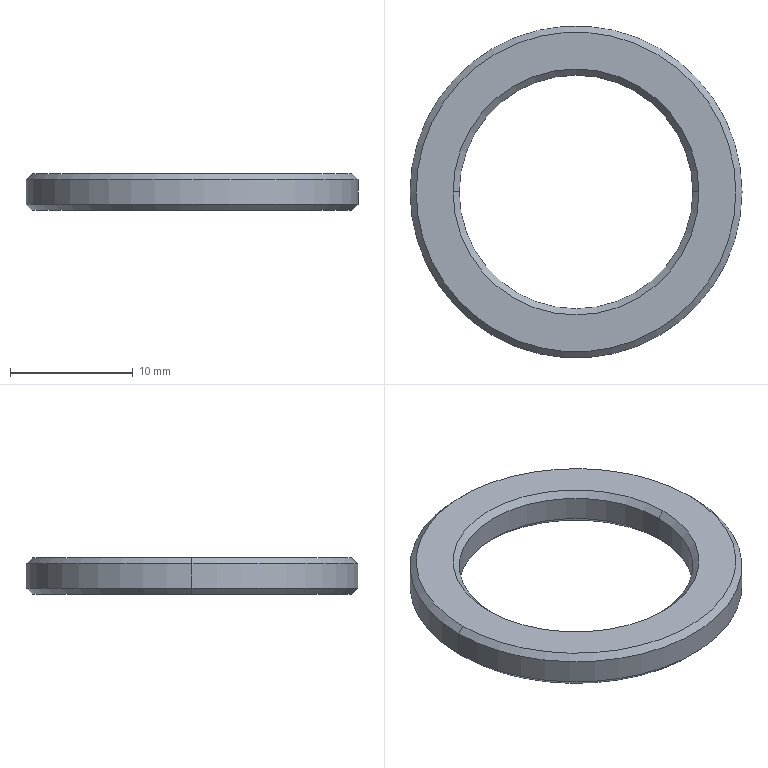Part | STEP file | FWSSS-D27-V19-T3-16 | 1 solid | 14 faces | box 27 x 27 x 3 mm | volume 830.951 mm3 | cone 8 | cylinder 4 | plane 2 | commonest cylinder face diameters 19 x2 27 x2
STEP:
#1=CARTESIAN_POINT('',(0.,0.,0.));
#2=DIRECTION('',(0.,0.,1.));
#3=DIRECTION('',(1.,0.,0.));
#4=AXIS2_PLACEMENT_3D('',#1,#2,#3);
#5=CARTESIAN_POINT('',(9.5,0.,-0.5));
#6=VERTEX_POINT('',#5);
#7=CARTESIAN_POINT('',(10.,0.,0.));
#8=VERTEX_POINT('',#7);
#9=CARTESIAN_POINT('',(10.,0.,0.));
#10=DIRECTION('',(0.7071,0.,0.7071));
#11=VECTOR('',#10,1.);
#12=LINE('',#9,#11);
#13=CARTESIAN_POINT('',(0.,0.,0.));
#14=DIRECTION('',(0.,0.,1.));
#15=DIRECTION('',(1.,0.,0.));
#16=AXIS2_PLACEMENT_3D('',#13,#14,#15);
#17=CONICAL_SURFACE('',#16,10.,0.7854);
#18=CARTESIAN_POINT('',(6.283,0.));
#19=DIRECTION('',(0.,1.));
#20=VECTOR('',#19,1.);
#21=LINE('',#18,#20);
#22=(GEOMETRIC_REPRESENTATION_CONTEXT(2)PARAMETRIC_REPRESENTATION_CONTEXT()REPRESENTATION_CONTEXT('',''));
#23=DEFINITIONAL_REPRESENTATION('',(#21),#22);
#24=PCURVE('',#17,#23);
#25=CARTESIAN_POINT('',(0.,0.,0.));
#26=DIRECTION('',(0.,0.,1.));
#27=DIRECTION('',(1.,0.,0.));
#28=AXIS2_PLACEMENT_3D('',#25,#26,#27);
#29=CONICAL_SURFACE('',#28,10.,0.7854);
#30=CARTESIAN_POINT('',(0.,0.));
#31=DIRECTION('',(0.,1.));
#32=VECTOR('',#31,1.);
#33=LINE('',#30,#32);
#34=(GEOMETRIC_REPRESENTATION_CONTEXT(2)PARAMETRIC_REPRESENTATION_CONTEXT()REPRESENTATION_CONTEXT('',''));
#35=DEFINITIONAL_REPRESENTATION('',(#33),#34);
#36=PCURVE('',#29,#35);
#37=SURFACE_CURVE('',#12,(#24,#36),.PCURVE_S1.);
#38=EDGE_CURVE('',#6,#8,#37,.T.);
#39=ORIENTED_EDGE('',*,*,#38,.T.);
#40=CARTESIAN_POINT('',(-10.,0.,0.));
#41=VERTEX_POINT('',#40);
#42=CARTESIAN_POINT('',(0.,0.,0.));
#43=DIRECTION('',(0.,0.,1.));
#44=DIRECTION('',(1.,0.,0.));
#45=AXIS2_PLACEMENT_3D('',#42,#43,#44);
#46=CIRCLE('',#45,10.);
#47=CARTESIAN_POINT('',(0.,0.));
#48=DIRECTION('',(1.,0.));
#49=VECTOR('',#48,1.);
#50=LINE('',#47,#49);
#51=(GEOMETRIC_REPRESENTATION_CONTEXT(2)PARAMETRIC_REPRESENTATION_CONTEXT()REPRESENTATION_CONTEXT('',''));
#52=DEFINITIONAL_REPRESENTATION('',(#50),#51);
#53=PCURVE('',#17,#52);
#54=CARTESIAN_POINT('',(13.5,0.,0.));
#55=DIRECTION('',(0.,0.,-1.));
#56=DIRECTION('',(-1.,0.,0.));
#57=AXIS2_PLACEMENT_3D('',#54,#55,#56);
#58=PLANE('',#57);
#59=CARTESIAN_POINT('',(3.5,0.));
#60=CARTESIAN_POINT('',(3.5,17.321));
#61=CARTESIAN_POINT('',(18.5,8.66));
#62=CARTESIAN_POINT('',(33.5,0.));
#63=CARTESIAN_POINT('',(18.5,-8.66));
#64=CARTESIAN_POINT('',(3.5,-17.321));
#65=CARTESIAN_POINT('',(3.5,0.));
#66=(BOUNDED_CURVE()B_SPLINE_CURVE(2,(#59,#60,#61,#62,#63,#64,#65),.UNSPECIFIED.,.T.,.F.)B_SPLINE_CURVE_WITH_KNOTS((1,2,2,2,2,1),(-2.094,0.,2.094,4.189,6.283,8.378),.UNSPECIFIED.)CURVE()GEOMETRIC_REPRESENTATION_ITEM()RATIONAL_B_SPLINE_CURVE((1.,0.5,1.,0.5,1.,0.5,1.))REPRESENTATION_ITEM(''));
#67=(GEOMETRIC_REPRESENTATION_CONTEXT(2)PARAMETRIC_REPRESENTATION_CONTEXT()REPRESENTATION_CONTEXT('',''));
#68=DEFINITIONAL_REPRESENTATION('',(#66),#67);
#69=PCURVE('',#58,#68);
#70=SURFACE_CURVE('',#46,(#53,#69),.PCURVE_S1.);
#71=EDGE_CURVE('',#41,#8,#70,.T.);
#72=ORIENTED_EDGE('',*,*,#71,.F.);
#73=CARTESIAN_POINT('',(-9.5,0.,-0.5));
#74=VERTEX_POINT('',#73);
#75=CARTESIAN_POINT('',(-10.,0.,0.));
#76=DIRECTION('',(-0.7071,0.,0.7071));
#77=VECTOR('',#76,1.);
#78=LINE('',#75,#77);
#79=CARTESIAN_POINT('',(3.142,0.));
#80=DIRECTION('',(0.,1.));
#81=VECTOR('',#80,1.);
#82=LINE('',#79,#81);
#83=(GEOMETRIC_REPRESENTATION_CONTEXT(2)PARAMETRIC_REPRESENTATION_CONTEXT()REPRESENTATION_CONTEXT('',''));
#84=DEFINITIONAL_REPRESENTATION('',(#82),#83);
#85=PCURVE('',#17,#84);
#86=CARTESIAN_POINT('',(3.142,0.));
#87=DIRECTION('',(0.,1.));
#88=VECTOR('',#87,1.);
#89=LINE('',#86,#88);
#90=(GEOMETRIC_REPRESENTATION_CONTEXT(2)PARAMETRIC_REPRESENTATION_CONTEXT()REPRESENTATION_CONTEXT('',''));
#91=DEFINITIONAL_REPRESENTATION('',(#89),#90);
#92=PCURVE('',#29,#91);
#93=SURFACE_CURVE('',#78,(#85,#92),.PCURVE_S1.);
#94=EDGE_CURVE('',#74,#41,#93,.T.);
#95=ORIENTED_EDGE('',*,*,#94,.F.);
#96=CARTESIAN_POINT('',(0.,0.,-0.5));
#97=DIRECTION('',(0.,0.,1.));
#98=DIRECTION('',(1.,0.,0.));
#99=AXIS2_PLACEMENT_3D('',#96,#97,#98);
#100=CIRCLE('',#99,9.5);
#101=CARTESIAN_POINT('',(0.,-0.5));
#102=DIRECTION('',(1.,0.));
#103=VECTOR('',#102,1.);
#104=LINE('',#101,#103);
#105=(GEOMETRIC_REPRESENTATION_CONTEXT(2)PARAMETRIC_REPRESENTATION_CONTEXT()REPRESENTATION_CONTEXT('',''));
#106=DEFINITIONAL_REPRESENTATION('',(#104),#105);
#107=PCURVE('',#17,#106);
#108=CARTESIAN_POINT('',(0.,0.,0.));
#109=DIRECTION('',(0.,0.,1.));
#110=DIRECTION('',(1.,0.,0.));
#111=AXIS2_PLACEMENT_3D('',#108,#109,#110);
#112=CYLINDRICAL_SURFACE('',#111,9.5);
#113=CARTESIAN_POINT('',(0.,-0.5));
#114=DIRECTION('',(1.,0.));
#115=VECTOR('',#114,1.);
#116=LINE('',#113,#115);
#117=(GEOMETRIC_REPRESENTATION_CONTEXT(2)PARAMETRIC_REPRESENTATION_CONTEXT()REPRESENTATION_CONTEXT('',''));
#118=DEFINITIONAL_REPRESENTATION('',(#116),#117);
#119=PCURVE('',#112,#118);
#120=SURFACE_CURVE('',#100,(#107,#119),.PCURVE_S1.);
#121=EDGE_CURVE('',#74,#6,#120,.T.);
#122=ORIENTED_EDGE('',*,*,#121,.T.);
#123=EDGE_LOOP('',(#39,#72,#95,#122));
#124=FACE_BOUND('',#123,.F.);
#125=ADVANCED_FACE('',(#124),#17,.F.);
#126=CARTESIAN_POINT('',(-9.5,0.,-2.5));
#127=VERTEX_POINT('',#126);
#128=CARTESIAN_POINT('',(-10.,0.,-3.));
#129=VERTEX_POINT('',#128);
#130=CARTESIAN_POINT('',(-9.5,0.,-2.5));
#131=DIRECTION('',(-0.7071,0.,-0.7071));
#132=VECTOR('',#131,1.);
#133=LINE('',#130,#132);
#134=CARTESIAN_POINT('',(0.,0.,-2.5));
#135=DIRECTION('',(0.,0.,-1.));
#136=DIRECTION('',(-1.,0.,0.));
#137=AXIS2_PLACEMENT_3D('',#134,#135,#136);
#138=CONICAL_SURFACE('',#137,9.5,0.7854);
#139=CARTESIAN_POINT('',(6.283,0.));
#140=DIRECTION('',(0.,1.));
#141=VECTOR('',#140,1.);
#142=LINE('',#139,#141);
#143=(GEOMETRIC_REPRESENTATION_CONTEXT(2)PARAMETRIC_REPRESENTATION_CONTEXT()REPRESENTATION_CONTEXT('',''));
#144=DEFINITIONAL_REPRESENTATION('',(#142),#143);
#145=PCURVE('',#138,#144);
#146=CARTESIAN_POINT('',(0.,0.,-2.5));
#147=DIRECTION('',(0.,0.,-1.));
#148=DIRECTION('',(-1.,0.,0.));
#149=AXIS2_PLACEMENT_3D('',#146,#147,#148);
#150=CONICAL_SURFACE('',#149,9.5,0.7854);
#151=CARTESIAN_POINT('',(0.,0.));
#152=DIRECTION('',(0.,1.));
#153=VECTOR('',#152,1.);
#154=LINE('',#151,#153);
#155=(GEOMETRIC_REPRESENTATION_CONTEXT(2)PARAMETRIC_REPRESENTATION_CONTEXT()REPRESENTATION_CONTEXT('',''));
#156=DEFINITIONAL_REPRESENTATION('',(#154),#155);
#157=PCURVE('',#150,#156);
#158=SURFACE_CURVE('',#133,(#145,#157),.PCURVE_S1.);
#159=EDGE_CURVE('',#127,#129,#158,.T.);
#160=ORIENTED_EDGE('',*,*,#159,.T.);
#161=CARTESIAN_POINT('',(10.,0.,-3.));
#162=VERTEX_POINT('',#161);
#163=CARTESIAN_POINT('',(0.,0.,-3.));
#164=DIRECTION('',(0.,0.,1.));
#165=DIRECTION('',(1.,0.,0.));
#166=AXIS2_PLACEMENT_3D('',#163,#164,#165);
#167=CIRCLE('',#166,10.);
#168=CARTESIAN_POINT('',(9.425,0.5));
#169=DIRECTION('',(-1.,0.));
#170=VECTOR('',#169,1.);
#171=LINE('',#168,#170);
#172=(GEOMETRIC_REPRESENTATION_CONTEXT(2)PARAMETRIC_REPRESENTATION_CONTEXT()REPRESENTATION_CONTEXT('',''));
#173=DEFINITIONAL_REPRESENTATION('',(#171),#172);
#174=PCURVE('',#138,#173);
#175=CARTESIAN_POINT('',(0.,0.,-3.));
#176=DIRECTION('',(0.,0.,1.));
#177=DIRECTION('',(1.,0.,0.));
#178=AXIS2_PLACEMENT_3D('',#175,#176,#177);
#179=PLANE('',#178);
#180=CARTESIAN_POINT('',(0.,0.));
#181=DIRECTION('',(1.,0.));
#182=AXIS2_PLACEMENT_2D('',#180,#181);
#183=CIRCLE('',#182,10.);
#184=(GEOMETRIC_REPRESENTATION_CONTEXT(2)PARAMETRIC_REPRESENTATION_CONTEXT()REPRESENTATION_CONTEXT('',''));
#185=DEFINITIONAL_REPRESENTATION('',(#183),#184);
#186=PCURVE('',#179,#185);
#187=SURFACE_CURVE('',#167,(#174,#186),.PCURVE_S1.);
#188=EDGE_CURVE('',#129,#162,#187,.T.);
#189=ORIENTED_EDGE('',*,*,#188,.T.);
#190=CARTESIAN_POINT('',(9.5,0.,-2.5));
#191=VERTEX_POINT('',#190);
#192=CARTESIAN_POINT('',(9.5,0.,-2.5));
#193=DIRECTION('',(0.7071,0.,-0.7071));
#194=VECTOR('',#193,1.);
#195=LINE('',#192,#194);
#196=CARTESIAN_POINT('',(3.142,0.));
#197=DIRECTION('',(0.,1.));
#198=VECTOR('',#197,1.);
#199=LINE('',#196,#198);
#200=(GEOMETRIC_REPRESENTATION_CONTEXT(2)PARAMETRIC_REPRESENTATION_CONTEXT()REPRESENTATION_CONTEXT('',''));
#201=DEFINITIONAL_REPRESENTATION('',(#199),#200);
#202=PCURVE('',#138,#201);
#203=CARTESIAN_POINT('',(3.142,0.));
#204=DIRECTION('',(0.,1.));
#205=VECTOR('',#204,1.);
#206=LINE('',#203,#205);
#207=(GEOMETRIC_REPRESENTATION_CONTEXT(2)PARAMETRIC_REPRESENTATION_CONTEXT()REPRESENTATION_CONTEXT('',''));
#208=DEFINITIONAL_REPRESENTATION('',(#206),#207);
#209=PCURVE('',#150,#208);
#210=SURFACE_CURVE('',#195,(#202,#209),.PCURVE_S1.);
#211=EDGE_CURVE('',#191,#162,#210,.T.);
#212=ORIENTED_EDGE('',*,*,#211,.F.);
#213=CARTESIAN_POINT('',(0.,0.,-2.5));
#214=DIRECTION('',(0.,0.,1.));
#215=DIRECTION('',(1.,0.,0.));
#216=AXIS2_PLACEMENT_3D('',#213,#214,#215);
#217=CIRCLE('',#216,9.5);
#218=CARTESIAN_POINT('',(9.425,0.));
#219=DIRECTION('',(-1.,0.));
#220=VECTOR('',#219,1.);
#221=LINE('',#218,#220);
#222=(GEOMETRIC_REPRESENTATION_CONTEXT(2)PARAMETRIC_REPRESENTATION_CONTEXT()REPRESENTATION_CONTEXT('',''));
#223=DEFINITIONAL_REPRESENTATION('',(#221),#222);
#224=PCURVE('',#138,#223);
#225=CARTESIAN_POINT('',(0.,-2.5));
#226=DIRECTION('',(1.,0.));
#227=VECTOR('',#226,1.);
#228=LINE('',#225,#227);
#229=(GEOMETRIC_REPRESENTATION_CONTEXT(2)PARAMETRIC_REPRESENTATION_CONTEXT()REPRESENTATION_CONTEXT('',''));
#230=DEFINITIONAL_REPRESENTATION('',(#228),#229);
#231=PCURVE('',#112,#230);
#232=SURFACE_CURVE('',#217,(#224,#231),.PCURVE_S1.);
#233=EDGE_CURVE('',#127,#191,#232,.T.);
#234=ORIENTED_EDGE('',*,*,#233,.F.);
#235=EDGE_LOOP('',(#160,#189,#212,#234));
#236=FACE_BOUND('',#235,.F.);
#237=ADVANCED_FACE('',(#236),#138,.F.);
#238=CARTESIAN_POINT('',(9.5,0.,0.));
#239=DIRECTION('',(0.,0.,1.));
#240=VECTOR('',#239,1.);
#241=LINE('',#238,#240);
#242=CARTESIAN_POINT('',(6.283,0.));
#243=DIRECTION('',(0.,1.));
#244=VECTOR('',#243,1.);
#245=LINE('',#242,#244);
#246=(GEOMETRIC_REPRESENTATION_CONTEXT(2)PARAMETRIC_REPRESENTATION_CONTEXT()REPRESENTATION_CONTEXT('',''));
#247=DEFINITIONAL_REPRESENTATION('',(#245),#246);
#248=PCURVE('',#112,#247);
#249=CARTESIAN_POINT('',(0.,0.,0.));
#250=DIRECTION('',(0.,0.,1.));
#251=DIRECTION('',(1.,0.,0.));
#252=AXIS2_PLACEMENT_3D('',#249,#250,#251);
#253=CYLINDRICAL_SURFACE('',#252,9.5);
#254=CARTESIAN_POINT('',(0.,0.));
#255=DIRECTION('',(0.,1.));
#256=VECTOR('',#255,1.);
#257=LINE('',#254,#256);
#258=(GEOMETRIC_REPRESENTATION_CONTEXT(2)PARAMETRIC_REPRESENTATION_CONTEXT()REPRESENTATION_CONTEXT('',''));
#259=DEFINITIONAL_REPRESENTATION('',(#257),#258);
#260=PCURVE('',#253,#259);
#261=SURFACE_CURVE('',#241,(#248,#260),.PCURVE_S1.);
#262=EDGE_CURVE('',#191,#6,#261,.T.);
#263=ORIENTED_EDGE('',*,*,#262,.T.);
#264=ORIENTED_EDGE('',*,*,#121,.F.);
#265=CARTESIAN_POINT('',(-9.5,0.,0.));
#266=DIRECTION('',(0.,0.,1.));
#267=VECTOR('',#266,1.);
#268=LINE('',#265,#267);
#269=CARTESIAN_POINT('',(3.142,0.));
#270=DIRECTION('',(0.,1.));
#271=VECTOR('',#270,1.);
#272=LINE('',#269,#271);
#273=(GEOMETRIC_REPRESENTATION_CONTEXT(2)PARAMETRIC_REPRESENTATION_CONTEXT()REPRESENTATION_CONTEXT('',''));
#274=DEFINITIONAL_REPRESENTATION('',(#272),#273);
#275=PCURVE('',#112,#274);
#276=CARTESIAN_POINT('',(3.142,0.));
#277=DIRECTION('',(0.,1.));
#278=VECTOR('',#277,1.);
#279=LINE('',#276,#278);
#280=(GEOMETRIC_REPRESENTATION_CONTEXT(2)PARAMETRIC_REPRESENTATION_CONTEXT()REPRESENTATION_CONTEXT('',''));
#281=DEFINITIONAL_REPRESENTATION('',(#279),#280);
#282=PCURVE('',#253,#281);
#283=SURFACE_CURVE('',#268,(#275,#282),.PCURVE_S1.);
#284=EDGE_CURVE('',#127,#74,#283,.T.);
#285=ORIENTED_EDGE('',*,*,#284,.F.);
#286=ORIENTED_EDGE('',*,*,#233,.T.);
#287=EDGE_LOOP('',(#263,#264,#285,#286));
#288=FACE_BOUND('',#287,.F.);
#289=ADVANCED_FACE('',(#288),#112,.F.);
#290=CARTESIAN_POINT('',(13.,0.,0.));
#291=VERTEX_POINT('',#290);
#292=CARTESIAN_POINT('',(-13.,0.,0.));
#293=VERTEX_POINT('',#292);
#294=CARTESIAN_POINT('',(0.,0.,0.));
#295=DIRECTION('',(0.,0.,1.));
#296=DIRECTION('',(1.,0.,0.));
#297=AXIS2_PLACEMENT_3D('',#294,#295,#296);
#298=CIRCLE('',#297,13.);
#299=CARTESIAN_POINT('',(0.,0.,-0.5));
#300=DIRECTION('',(0.,0.,-1.));
#301=DIRECTION('',(-1.,0.,0.));
#302=AXIS2_PLACEMENT_3D('',#299,#300,#301);
#303=CONICAL_SURFACE('',#302,13.5,0.7854);
#304=CARTESIAN_POINT('',(3.142,-0.5));
#305=DIRECTION('',(-1.,0.));
#306=VECTOR('',#305,1.);
#307=LINE('',#304,#306);
#308=(GEOMETRIC_REPRESENTATION_CONTEXT(2)PARAMETRIC_REPRESENTATION_CONTEXT()REPRESENTATION_CONTEXT('',''));
#309=DEFINITIONAL_REPRESENTATION('',(#307),#308);
#310=PCURVE('',#303,#309);
#311=CARTESIAN_POINT('',(0.5,0.));
#312=CARTESIAN_POINT('',(0.5,22.517));
#313=CARTESIAN_POINT('',(20.,11.258));
#314=CARTESIAN_POINT('',(39.5,0.));
#315=CARTESIAN_POINT('',(20.,-11.258));
#316=CARTESIAN_POINT('',(0.5,-22.517));
#317=CARTESIAN_POINT('',(0.5,0.));
#318=(BOUNDED_CURVE()B_SPLINE_CURVE(2,(#311,#312,#313,#314,#315,#316,#317),.UNSPECIFIED.,.T.,.F.)B_SPLINE_CURVE_WITH_KNOTS((1,2,2,2,2,1),(-2.094,0.,2.094,4.189,6.283,8.378),.UNSPECIFIED.)CURVE()GEOMETRIC_REPRESENTATION_ITEM()RATIONAL_B_SPLINE_CURVE((1.,0.5,1.,0.5,1.,0.5,1.))REPRESENTATION_ITEM(''));
#319=(GEOMETRIC_REPRESENTATION_CONTEXT(2)PARAMETRIC_REPRESENTATION_CONTEXT()REPRESENTATION_CONTEXT('',''));
#320=DEFINITIONAL_REPRESENTATION('',(#318),#319);
#321=PCURVE('',#58,#320);
#322=SURFACE_CURVE('',#298,(#310,#321),.PCURVE_S1.);
#323=EDGE_CURVE('',#291,#293,#322,.T.);
#324=ORIENTED_EDGE('',*,*,#323,.F.);
#325=CARTESIAN_POINT('',(13.5,0.,-0.5));
#326=VERTEX_POINT('',#325);
#327=CARTESIAN_POINT('',(13.5,0.,-0.5));
#328=DIRECTION('',(0.7071,0.,-0.7071));
#329=VECTOR('',#328,1.);
#330=LINE('',#327,#329);
#331=CARTESIAN_POINT('',(3.142,0.));
#332=DIRECTION('',(0.,1.));
#333=VECTOR('',#332,1.);
#334=LINE('',#331,#333);
#335=(GEOMETRIC_REPRESENTATION_CONTEXT(2)PARAMETRIC_REPRESENTATION_CONTEXT()REPRESENTATION_CONTEXT('',''));
#336=DEFINITIONAL_REPRESENTATION('',(#334),#335);
#337=PCURVE('',#303,#336);
#338=CARTESIAN_POINT('',(0.,0.,-0.5));
#339=DIRECTION('',(0.,0.,-1.));
#340=DIRECTION('',(-1.,0.,0.));
#341=AXIS2_PLACEMENT_3D('',#338,#339,#340);
#342=CONICAL_SURFACE('',#341,13.5,0.7854);
#343=CARTESIAN_POINT('',(3.142,0.));
#344=DIRECTION('',(0.,1.));
#345=VECTOR('',#344,1.);
#346=LINE('',#343,#345);
#347=(GEOMETRIC_REPRESENTATION_CONTEXT(2)PARAMETRIC_REPRESENTATION_CONTEXT()REPRESENTATION_CONTEXT('',''));
#348=DEFINITIONAL_REPRESENTATION('',(#346),#347);
#349=PCURVE('',#342,#348);
#350=SURFACE_CURVE('',#330,(#337,#349),.PCURVE_S1.);
#351=EDGE_CURVE('',#291,#326,#350,.T.);
#352=ORIENTED_EDGE('',*,*,#351,.T.);
#353=CARTESIAN_POINT('',(-13.5,0.,-0.5));
#354=VERTEX_POINT('',#353);
#355=CARTESIAN_POINT('',(0.,0.,-0.5));
#356=DIRECTION('',(0.,0.,1.));
#357=DIRECTION('',(1.,0.,0.));
#358=AXIS2_PLACEMENT_3D('',#355,#356,#357);
#359=CIRCLE('',#358,13.5);
#360=CARTESIAN_POINT('',(3.142,0.));
#361=DIRECTION('',(-1.,0.));
#362=VECTOR('',#361,1.);
#363=LINE('',#360,#362);
#364=(GEOMETRIC_REPRESENTATION_CONTEXT(2)PARAMETRIC_REPRESENTATION_CONTEXT()REPRESENTATION_CONTEXT('',''));
#365=DEFINITIONAL_REPRESENTATION('',(#363),#364);
#366=PCURVE('',#303,#365);
#367=CARTESIAN_POINT('',(0.,0.,0.));
#368=DIRECTION('',(0.,0.,1.));
#369=DIRECTION('',(1.,0.,0.));
#370=AXIS2_PLACEMENT_3D('',#367,#368,#369);
#371=CYLINDRICAL_SURFACE('',#370,13.5);
#372=CARTESIAN_POINT('',(0.,-0.5));
#373=DIRECTION('',(1.,0.));
#374=VECTOR('',#373,1.);
#375=LINE('',#372,#374);
#376=(GEOMETRIC_REPRESENTATION_CONTEXT(2)PARAMETRIC_REPRESENTATION_CONTEXT()REPRESENTATION_CONTEXT('',''));
#377=DEFINITIONAL_REPRESENTATION('',(#375),#376);
#378=PCURVE('',#371,#377);
#379=SURFACE_CURVE('',#359,(#366,#378),.PCURVE_S1.);
#380=EDGE_CURVE('',#326,#354,#379,.T.);
#381=ORIENTED_EDGE('',*,*,#380,.T.);
#382=CARTESIAN_POINT('',(-13.5,0.,-0.5));
#383=DIRECTION('',(-0.7071,0.,-0.7071));
#384=VECTOR('',#383,1.);
#385=LINE('',#382,#384);
#386=CARTESIAN_POINT('',(0.,0.));
#387=DIRECTION('',(0.,1.));
#388=VECTOR('',#387,1.);
#389=LINE('',#386,#388);
#390=(GEOMETRIC_REPRESENTATION_CONTEXT(2)PARAMETRIC_REPRESENTATION_CONTEXT()REPRESENTATION_CONTEXT('',''));
#391=DEFINITIONAL_REPRESENTATION('',(#389),#390);
#392=PCURVE('',#303,#391);
#393=CARTESIAN_POINT('',(6.283,0.));
#394=DIRECTION('',(0.,1.));
#395=VECTOR('',#394,1.);
#396=LINE('',#393,#395);
#397=(GEOMETRIC_REPRESENTATION_CONTEXT(2)PARAMETRIC_REPRESENTATION_CONTEXT()REPRESENTATION_CONTEXT('',''));
#398=DEFINITIONAL_REPRESENTATION('',(#396),#397);
#399=PCURVE('',#342,#398);
#400=SURFACE_CURVE('',#385,(#392,#399),.PCURVE_S1.);
#401=EDGE_CURVE('',#293,#354,#400,.T.);
#402=ORIENTED_EDGE('',*,*,#401,.F.);
#403=EDGE_LOOP('',(#324,#352,#381,#402));
#404=FACE_BOUND('',#403,.T.);
#405=ADVANCED_FACE('',(#404),#303,.T.);
#406=CARTESIAN_POINT('',(13.,0.,-3.));
#407=VERTEX_POINT('',#406);
#408=CARTESIAN_POINT('',(-13.,0.,-3.));
#409=VERTEX_POINT('',#408);
#410=CARTESIAN_POINT('',(0.,0.,-3.));
#411=DIRECTION('',(0.,0.,1.));
#412=DIRECTION('',(1.,0.,0.));
#413=AXIS2_PLACEMENT_3D('',#410,#411,#412);
#414=CIRCLE('',#413,13.);
#415=CARTESIAN_POINT('',(0.,0.,-3.));
#416=DIRECTION('',(0.,0.,1.));
#417=DIRECTION('',(1.,0.,0.));
#418=AXIS2_PLACEMENT_3D('',#415,#416,#417);
#419=CONICAL_SURFACE('',#418,13.,0.7854);
#420=CARTESIAN_POINT('',(0.,0.));
#421=DIRECTION('',(1.,0.));
#422=VECTOR('',#421,1.);
#423=LINE('',#420,#422);
#424=(GEOMETRIC_REPRESENTATION_CONTEXT(2)PARAMETRIC_REPRESENTATION_CONTEXT()REPRESENTATION_CONTEXT('',''));
#425=DEFINITIONAL_REPRESENTATION('',(#423),#424);
#426=PCURVE('',#419,#425);
#427=CARTESIAN_POINT('',(0.,0.));
#428=DIRECTION('',(1.,0.));
#429=AXIS2_PLACEMENT_2D('',#427,#428);
#430=CIRCLE('',#429,13.);
#431=(GEOMETRIC_REPRESENTATION_CONTEXT(2)PARAMETRIC_REPRESENTATION_CONTEXT()REPRESENTATION_CONTEXT('',''));
#432=DEFINITIONAL_REPRESENTATION('',(#430),#431);
#433=PCURVE('',#179,#432);
#434=SURFACE_CURVE('',#414,(#426,#433),.PCURVE_S1.);
#435=EDGE_CURVE('',#407,#409,#434,.T.);
#436=ORIENTED_EDGE('',*,*,#435,.T.);
#437=CARTESIAN_POINT('',(-13.5,0.,-2.5));
#438=VERTEX_POINT('',#437);
#439=CARTESIAN_POINT('',(-13.,0.,-3.));
#440=DIRECTION('',(-0.7071,0.,0.7071));
#441=VECTOR('',#440,1.);
#442=LINE('',#439,#441);
#443=CARTESIAN_POINT('',(3.142,0.));
#444=DIRECTION('',(0.,1.));
#445=VECTOR('',#444,1.);
#446=LINE('',#443,#445);
#447=(GEOMETRIC_REPRESENTATION_CONTEXT(2)PARAMETRIC_REPRESENTATION_CONTEXT()REPRESENTATION_CONTEXT('',''));
#448=DEFINITIONAL_REPRESENTATION('',(#446),#447);
#449=PCURVE('',#419,#448);
#450=CARTESIAN_POINT('',(0.,0.,-3.));
#451=DIRECTION('',(0.,0.,1.));
#452=DIRECTION('',(1.,0.,0.));
#453=AXIS2_PLACEMENT_3D('',#450,#451,#452);
#454=CONICAL_SURFACE('',#453,13.,0.7854);
#455=CARTESIAN_POINT('',(3.142,0.));
#456=DIRECTION('',(0.,1.));
#457=VECTOR('',#456,1.);
#458=LINE('',#455,#457);
#459=(GEOMETRIC_REPRESENTATION_CONTEXT(2)PARAMETRIC_REPRESENTATION_CONTEXT()REPRESENTATION_CONTEXT('',''));
#460=DEFINITIONAL_REPRESENTATION('',(#458),#459);
#461=PCURVE('',#454,#460);
#462=SURFACE_CURVE('',#442,(#449,#461),.PCURVE_S1.);
#463=EDGE_CURVE('',#409,#438,#462,.T.);
#464=ORIENTED_EDGE('',*,*,#463,.T.);
#465=CARTESIAN_POINT('',(13.5,0.,-2.5));
#466=VERTEX_POINT('',#465);
#467=CARTESIAN_POINT('',(0.,0.,-2.5));
#468=DIRECTION('',(0.,0.,1.));
#469=DIRECTION('',(1.,0.,0.));
#470=AXIS2_PLACEMENT_3D('',#467,#468,#469);
#471=CIRCLE('',#470,13.5);
#472=CARTESIAN_POINT('',(0.,0.5));
#473=DIRECTION('',(1.,0.));
#474=VECTOR('',#473,1.);
#475=LINE('',#472,#474);
#476=(GEOMETRIC_REPRESENTATION_CONTEXT(2)PARAMETRIC_REPRESENTATION_CONTEXT()REPRESENTATION_CONTEXT('',''));
#477=DEFINITIONAL_REPRESENTATION('',(#475),#476);
#478=PCURVE('',#419,#477);
#479=CARTESIAN_POINT('',(0.,-2.5));
#480=DIRECTION('',(1.,0.));
#481=VECTOR('',#480,1.);
#482=LINE('',#479,#481);
#483=(GEOMETRIC_REPRESENTATION_CONTEXT(2)PARAMETRIC_REPRESENTATION_CONTEXT()REPRESENTATION_CONTEXT('',''));
#484=DEFINITIONAL_REPRESENTATION('',(#482),#483);
#485=PCURVE('',#371,#484);
#486=SURFACE_CURVE('',#471,(#478,#485),.PCURVE_S1.);
#487=EDGE_CURVE('',#466,#438,#486,.T.);
#488=ORIENTED_EDGE('',*,*,#487,.F.);
#489=CARTESIAN_POINT('',(13.,0.,-3.));
#490=DIRECTION('',(0.7071,0.,0.7071));
#491=VECTOR('',#490,1.);
#492=LINE('',#489,#491);
#493=CARTESIAN_POINT('',(0.,0.));
#494=DIRECTION('',(0.,1.));
#495=VECTOR('',#494,1.);
#496=LINE('',#493,#495);
#497=(GEOMETRIC_REPRESENTATION_CONTEXT(2)PARAMETRIC_REPRESENTATION_CONTEXT()REPRESENTATION_CONTEXT('',''));
#498=DEFINITIONAL_REPRESENTATION('',(#496),#497);
#499=PCURVE('',#419,#498);
#500=CARTESIAN_POINT('',(6.283,0.));
#501=DIRECTION('',(0.,1.));
#502=VECTOR('',#501,1.);
#503=LINE('',#500,#502);
#504=(GEOMETRIC_REPRESENTATION_CONTEXT(2)PARAMETRIC_REPRESENTATION_CONTEXT()REPRESENTATION_CONTEXT('',''));
#505=DEFINITIONAL_REPRESENTATION('',(#503),#504);
#506=PCURVE('',#454,#505);
#507=SURFACE_CURVE('',#492,(#499,#506),.PCURVE_S1.);
#508=EDGE_CURVE('',#407,#466,#507,.T.);
#509=ORIENTED_EDGE('',*,*,#508,.F.);
#510=EDGE_LOOP('',(#436,#464,#488,#509));
#511=FACE_BOUND('',#510,.T.);
#512=ADVANCED_FACE('',(#511),#419,.T.);
#513=ORIENTED_EDGE('',*,*,#487,.T.);
#514=CARTESIAN_POINT('',(-13.5,0.,0.));
#515=DIRECTION('',(0.,0.,1.));
#516=VECTOR('',#515,1.);
#517=LINE('',#514,#516);
#518=CARTESIAN_POINT('',(3.142,0.));
#519=DIRECTION('',(0.,1.));
#520=VECTOR('',#519,1.);
#521=LINE('',#518,#520);
#522=(GEOMETRIC_REPRESENTATION_CONTEXT(2)PARAMETRIC_REPRESENTATION_CONTEXT()REPRESENTATION_CONTEXT('',''));
#523=DEFINITIONAL_REPRESENTATION('',(#521),#522);
#524=PCURVE('',#371,#523);
#525=CARTESIAN_POINT('',(0.,0.,0.));
#526=DIRECTION('',(0.,0.,1.));
#527=DIRECTION('',(1.,0.,0.));
#528=AXIS2_PLACEMENT_3D('',#525,#526,#527);
#529=CYLINDRICAL_SURFACE('',#528,13.5);
#530=CARTESIAN_POINT('',(3.142,0.));
#531=DIRECTION('',(0.,1.));
#532=VECTOR('',#531,1.);
#533=LINE('',#530,#532);
#534=(GEOMETRIC_REPRESENTATION_CONTEXT(2)PARAMETRIC_REPRESENTATION_CONTEXT()REPRESENTATION_CONTEXT('',''));
#535=DEFINITIONAL_REPRESENTATION('',(#533),#534);
#536=PCURVE('',#529,#535);
#537=SURFACE_CURVE('',#517,(#524,#536),.PCURVE_S1.);
#538=EDGE_CURVE('',#438,#354,#537,.T.);
#539=ORIENTED_EDGE('',*,*,#538,.T.);
#540=ORIENTED_EDGE('',*,*,#380,.F.);
#541=CARTESIAN_POINT('',(13.5,0.,0.));
#542=DIRECTION('',(0.,0.,1.));
#543=VECTOR('',#542,1.);
#544=LINE('',#541,#543);
#545=CARTESIAN_POINT('',(0.,0.));
#546=DIRECTION('',(0.,1.));
#547=VECTOR('',#546,1.);
#548=LINE('',#545,#547);
#549=(GEOMETRIC_REPRESENTATION_CONTEXT(2)PARAMETRIC_REPRESENTATION_CONTEXT()REPRESENTATION_CONTEXT('',''));
#550=DEFINITIONAL_REPRESENTATION('',(#548),#549);
#551=PCURVE('',#371,#550);
#552=CARTESIAN_POINT('',(6.283,0.));
#553=DIRECTION('',(0.,1.));
#554=VECTOR('',#553,1.);
#555=LINE('',#552,#554);
#556=(GEOMETRIC_REPRESENTATION_CONTEXT(2)PARAMETRIC_REPRESENTATION_CONTEXT()REPRESENTATION_CONTEXT('',''));
#557=DEFINITIONAL_REPRESENTATION('',(#555),#556);
#558=PCURVE('',#529,#557);
#559=SURFACE_CURVE('',#544,(#551,#558),.PCURVE_S1.);
#560=EDGE_CURVE('',#466,#326,#559,.T.);
#561=ORIENTED_EDGE('',*,*,#560,.F.);
#562=EDGE_LOOP('',(#513,#539,#540,#561));
#563=FACE_BOUND('',#562,.T.);
#564=ADVANCED_FACE('',(#563),#371,.T.);
#565=ORIENTED_EDGE('',*,*,#538,.F.);
#566=CARTESIAN_POINT('',(0.,0.,-2.5));
#567=DIRECTION('',(0.,0.,1.));
#568=DIRECTION('',(1.,0.,0.));
#569=AXIS2_PLACEMENT_3D('',#566,#567,#568);
#570=CIRCLE('',#569,13.5);
#571=CARTESIAN_POINT('',(0.,-2.5));
#572=DIRECTION('',(1.,0.));
#573=VECTOR('',#572,1.);
#574=LINE('',#571,#573);
#575=(GEOMETRIC_REPRESENTATION_CONTEXT(2)PARAMETRIC_REPRESENTATION_CONTEXT()REPRESENTATION_CONTEXT('',''));
#576=DEFINITIONAL_REPRESENTATION('',(#574),#575);
#577=PCURVE('',#529,#576);
#578=CARTESIAN_POINT('',(0.,0.5));
#579=DIRECTION('',(1.,0.));
#580=VECTOR('',#579,1.);
#581=LINE('',#578,#580);
#582=(GEOMETRIC_REPRESENTATION_CONTEXT(2)PARAMETRIC_REPRESENTATION_CONTEXT()REPRESENTATION_CONTEXT('',''));
#583=DEFINITIONAL_REPRESENTATION('',(#581),#582);
#584=PCURVE('',#454,#583);
#585=SURFACE_CURVE('',#570,(#577,#584),.PCURVE_S1.);
#586=EDGE_CURVE('',#438,#466,#585,.T.);
#587=ORIENTED_EDGE('',*,*,#586,.T.);
#588=ORIENTED_EDGE('',*,*,#560,.T.);
#589=CARTESIAN_POINT('',(0.,0.,-0.5));
#590=DIRECTION('',(0.,0.,1.));
#591=DIRECTION('',(1.,0.,0.));
#592=AXIS2_PLACEMENT_3D('',#589,#590,#591);
#593=CIRCLE('',#592,13.5);
#594=CARTESIAN_POINT('',(0.,-0.5));
#595=DIRECTION('',(1.,0.));
#596=VECTOR('',#595,1.);
#597=LINE('',#594,#596);
#598=(GEOMETRIC_REPRESENTATION_CONTEXT(2)PARAMETRIC_REPRESENTATION_CONTEXT()REPRESENTATION_CONTEXT('',''));
#599=DEFINITIONAL_REPRESENTATION('',(#597),#598);
#600=PCURVE('',#529,#599);
#601=CARTESIAN_POINT('',(9.425,0.));
#602=DIRECTION('',(-1.,0.));
#603=VECTOR('',#602,1.);
#604=LINE('',#601,#603);
#605=(GEOMETRIC_REPRESENTATION_CONTEXT(2)PARAMETRIC_REPRESENTATION_CONTEXT()REPRESENTATION_CONTEXT('',''));
#606=DEFINITIONAL_REPRESENTATION('',(#604),#605);
#607=PCURVE('',#342,#606);
#608=SURFACE_CURVE('',#593,(#600,#607),.PCURVE_S1.);
#609=EDGE_CURVE('',#354,#326,#608,.T.);
#610=ORIENTED_EDGE('',*,*,#609,.F.);
#611=EDGE_LOOP('',(#565,#587,#588,#610));
#612=FACE_BOUND('',#611,.T.);
#613=ADVANCED_FACE('',(#612),#529,.T.);
#614=ORIENTED_EDGE('',*,*,#463,.F.);
#615=CARTESIAN_POINT('',(0.,0.,-3.));
#616=DIRECTION('',(0.,0.,1.));
#617=DIRECTION('',(1.,0.,0.));
#618=AXIS2_PLACEMENT_3D('',#615,#616,#617);
#619=CIRCLE('',#618,13.);
#620=CARTESIAN_POINT('',(0.,0.));
#621=DIRECTION('',(1.,0.));
#622=VECTOR('',#621,1.);
#623=LINE('',#620,#622);
#624=(GEOMETRIC_REPRESENTATION_CONTEXT(2)PARAMETRIC_REPRESENTATION_CONTEXT()REPRESENTATION_CONTEXT('',''));
#625=DEFINITIONAL_REPRESENTATION('',(#623),#624);
#626=PCURVE('',#454,#625);
#627=CARTESIAN_POINT('',(0.,0.));
#628=DIRECTION('',(1.,0.));
#629=AXIS2_PLACEMENT_2D('',#627,#628);
#630=CIRCLE('',#629,13.);
#631=(GEOMETRIC_REPRESENTATION_CONTEXT(2)PARAMETRIC_REPRESENTATION_CONTEXT()REPRESENTATION_CONTEXT('',''));
#632=DEFINITIONAL_REPRESENTATION('',(#630),#631);
#633=PCURVE('',#179,#632);
#634=SURFACE_CURVE('',#619,(#626,#633),.PCURVE_S1.);
#635=EDGE_CURVE('',#409,#407,#634,.T.);
#636=ORIENTED_EDGE('',*,*,#635,.T.);
#637=ORIENTED_EDGE('',*,*,#508,.T.);
#638=ORIENTED_EDGE('',*,*,#586,.F.);
#639=EDGE_LOOP('',(#614,#636,#637,#638));
#640=FACE_BOUND('',#639,.T.);
#641=ADVANCED_FACE('',(#640),#454,.T.);
#642=ORIENTED_EDGE('',*,*,#435,.F.);
#643=ORIENTED_EDGE('',*,*,#635,.F.);
#644=EDGE_LOOP('',(#642,#643));
#645=FACE_BOUND('',#644,.T.);
#646=ORIENTED_EDGE('',*,*,#188,.T.);
#647=CARTESIAN_POINT('',(0.,0.,-3.));
#648=DIRECTION('',(0.,0.,1.));
#649=DIRECTION('',(1.,0.,0.));
#650=AXIS2_PLACEMENT_3D('',#647,#648,#649);
#651=CIRCLE('',#650,10.);
#652=CARTESIAN_POINT('',(0.,0.));
#653=DIRECTION('',(1.,0.));
#654=AXIS2_PLACEMENT_2D('',#652,#653);
#655=CIRCLE('',#654,10.);
#656=(GEOMETRIC_REPRESENTATION_CONTEXT(2)PARAMETRIC_REPRESENTATION_CONTEXT()REPRESENTATION_CONTEXT('',''));
#657=DEFINITIONAL_REPRESENTATION('',(#655),#656);
#658=PCURVE('',#179,#657);
#659=CARTESIAN_POINT('',(3.142,0.5));
#660=DIRECTION('',(-1.,0.));
#661=VECTOR('',#660,1.);
#662=LINE('',#659,#661);
#663=(GEOMETRIC_REPRESENTATION_CONTEXT(2)PARAMETRIC_REPRESENTATION_CONTEXT()REPRESENTATION_CONTEXT('',''));
#664=DEFINITIONAL_REPRESENTATION('',(#662),#663);
#665=PCURVE('',#150,#664);
#666=SURFACE_CURVE('',#651,(#658,#665),.PCURVE_S1.);
#667=EDGE_CURVE('',#162,#129,#666,.T.);
#668=ORIENTED_EDGE('',*,*,#667,.T.);
#669=EDGE_LOOP('',(#646,#668));
#670=FACE_BOUND('',#669,.T.);
#671=ADVANCED_FACE('',(#645,#670),#179,.F.);
#672=ORIENTED_EDGE('',*,*,#351,.F.);
#673=CARTESIAN_POINT('',(0.,0.,0.));
#674=DIRECTION('',(0.,0.,1.));
#675=DIRECTION('',(1.,0.,0.));
#676=AXIS2_PLACEMENT_3D('',#673,#674,#675);
#677=CIRCLE('',#676,13.);
#678=CARTESIAN_POINT('',(9.425,-0.5));
#679=DIRECTION('',(-1.,0.));
#680=VECTOR('',#679,1.);
#681=LINE('',#678,#680);
#682=(GEOMETRIC_REPRESENTATION_CONTEXT(2)PARAMETRIC_REPRESENTATION_CONTEXT()REPRESENTATION_CONTEXT('',''));
#683=DEFINITIONAL_REPRESENTATION('',(#681),#682);
#684=PCURVE('',#342,#683);
#685=CARTESIAN_POINT('',(0.5,0.));
#686=CARTESIAN_POINT('',(0.5,22.517));
#687=CARTESIAN_POINT('',(20.,11.258));
#688=CARTESIAN_POINT('',(39.5,0.));
#689=CARTESIAN_POINT('',(20.,-11.258));
#690=CARTESIAN_POINT('',(0.5,-22.517));
#691=CARTESIAN_POINT('',(0.5,0.));
#692=(BOUNDED_CURVE()B_SPLINE_CURVE(2,(#685,#686,#687,#688,#689,#690,#691),.UNSPECIFIED.,.T.,.F.)B_SPLINE_CURVE_WITH_KNOTS((1,2,2,2,2,1),(-2.094,0.,2.094,4.189,6.283,8.378),.UNSPECIFIED.)CURVE()GEOMETRIC_REPRESENTATION_ITEM()RATIONAL_B_SPLINE_CURVE((1.,0.5,1.,0.5,1.,0.5,1.))REPRESENTATION_ITEM(''));
#693=(GEOMETRIC_REPRESENTATION_CONTEXT(2)PARAMETRIC_REPRESENTATION_CONTEXT()REPRESENTATION_CONTEXT('',''));
#694=DEFINITIONAL_REPRESENTATION('',(#692),#693);
#695=PCURVE('',#58,#694);
#696=SURFACE_CURVE('',#677,(#684,#695),.PCURVE_S1.);
#697=EDGE_CURVE('',#293,#291,#696,.T.);
#698=ORIENTED_EDGE('',*,*,#697,.F.);
#699=ORIENTED_EDGE('',*,*,#401,.T.);
#700=ORIENTED_EDGE('',*,*,#609,.T.);
#701=EDGE_LOOP('',(#672,#698,#699,#700));
#702=FACE_BOUND('',#701,.T.);
#703=ADVANCED_FACE('',(#702),#342,.T.);
#704=CARTESIAN_POINT('',(0.,0.,0.));
#705=DIRECTION('',(0.,0.,1.));
#706=DIRECTION('',(1.,0.,0.));
#707=AXIS2_PLACEMENT_3D('',#704,#705,#706);
#708=CIRCLE('',#707,10.);
#709=CARTESIAN_POINT('',(3.5,0.));
#710=CARTESIAN_POINT('',(3.5,17.321));
#711=CARTESIAN_POINT('',(18.5,8.66));
#712=CARTESIAN_POINT('',(33.5,0.));
#713=CARTESIAN_POINT('',(18.5,-8.66));
#714=CARTESIAN_POINT('',(3.5,-17.321));
#715=CARTESIAN_POINT('',(3.5,0.));
#716=(BOUNDED_CURVE()B_SPLINE_CURVE(2,(#709,#710,#711,#712,#713,#714,#715),.UNSPECIFIED.,.T.,.F.)B_SPLINE_CURVE_WITH_KNOTS((1,2,2,2,2,1),(-2.094,0.,2.094,4.189,6.283,8.378),.UNSPECIFIED.)CURVE()GEOMETRIC_REPRESENTATION_ITEM()RATIONAL_B_SPLINE_CURVE((1.,0.5,1.,0.5,1.,0.5,1.))REPRESENTATION_ITEM(''));
#717=(GEOMETRIC_REPRESENTATION_CONTEXT(2)PARAMETRIC_REPRESENTATION_CONTEXT()REPRESENTATION_CONTEXT('',''));
#718=DEFINITIONAL_REPRESENTATION('',(#716),#717);
#719=PCURVE('',#58,#718);
#720=CARTESIAN_POINT('',(0.,0.));
#721=DIRECTION('',(1.,0.));
#722=VECTOR('',#721,1.);
#723=LINE('',#720,#722);
#724=(GEOMETRIC_REPRESENTATION_CONTEXT(2)PARAMETRIC_REPRESENTATION_CONTEXT()REPRESENTATION_CONTEXT('',''));
#725=DEFINITIONAL_REPRESENTATION('',(#723),#724);
#726=PCURVE('',#29,#725);
#727=SURFACE_CURVE('',#708,(#719,#726),.PCURVE_S1.);
#728=EDGE_CURVE('',#8,#41,#727,.T.);
#729=ORIENTED_EDGE('',*,*,#728,.F.);
#730=ORIENTED_EDGE('',*,*,#71,.F.);
#731=EDGE_LOOP('',(#729,#730));
#732=FACE_BOUND('',#731,.T.);
#733=ORIENTED_EDGE('',*,*,#697,.T.);
#734=ORIENTED_EDGE('',*,*,#323,.T.);
#735=EDGE_LOOP('',(#733,#734));
#736=FACE_BOUND('',#735,.T.);
#737=ADVANCED_FACE('',(#732,#736),#58,.F.);
#738=CARTESIAN_POINT('',(0.,0.,-0.5));
#739=DIRECTION('',(0.,0.,1.));
#740=DIRECTION('',(1.,0.,0.));
#741=AXIS2_PLACEMENT_3D('',#738,#739,#740);
#742=CIRCLE('',#741,9.5);
#743=CARTESIAN_POINT('',(0.,-0.5));
#744=DIRECTION('',(1.,0.));
#745=VECTOR('',#744,1.);
#746=LINE('',#743,#745);
#747=(GEOMETRIC_REPRESENTATION_CONTEXT(2)PARAMETRIC_REPRESENTATION_CONTEXT()REPRESENTATION_CONTEXT('',''));
#748=DEFINITIONAL_REPRESENTATION('',(#746),#747);
#749=PCURVE('',#253,#748);
#750=CARTESIAN_POINT('',(0.,-0.5));
#751=DIRECTION('',(1.,0.));
#752=VECTOR('',#751,1.);
#753=LINE('',#750,#752);
#754=(GEOMETRIC_REPRESENTATION_CONTEXT(2)PARAMETRIC_REPRESENTATION_CONTEXT()REPRESENTATION_CONTEXT('',''));
#755=DEFINITIONAL_REPRESENTATION('',(#753),#754);
#756=PCURVE('',#29,#755);
#757=SURFACE_CURVE('',#742,(#749,#756),.PCURVE_S1.);
#758=EDGE_CURVE('',#6,#74,#757,.T.);
#759=ORIENTED_EDGE('',*,*,#758,.F.);
#760=ORIENTED_EDGE('',*,*,#262,.F.);
#761=CARTESIAN_POINT('',(0.,0.,-2.5));
#762=DIRECTION('',(0.,0.,1.));
#763=DIRECTION('',(1.,0.,0.));
#764=AXIS2_PLACEMENT_3D('',#761,#762,#763);
#765=CIRCLE('',#764,9.5);
#766=CARTESIAN_POINT('',(0.,-2.5));
#767=DIRECTION('',(1.,0.));
#768=VECTOR('',#767,1.);
#769=LINE('',#766,#768);
#770=(GEOMETRIC_REPRESENTATION_CONTEXT(2)PARAMETRIC_REPRESENTATION_CONTEXT()REPRESENTATION_CONTEXT('',''));
#771=DEFINITIONAL_REPRESENTATION('',(#769),#770);
#772=PCURVE('',#253,#771);
#773=CARTESIAN_POINT('',(3.142,0.));
#774=DIRECTION('',(-1.,0.));
#775=VECTOR('',#774,1.);
#776=LINE('',#773,#775);
#777=(GEOMETRIC_REPRESENTATION_CONTEXT(2)PARAMETRIC_REPRESENTATION_CONTEXT()REPRESENTATION_CONTEXT('',''));
#778=DEFINITIONAL_REPRESENTATION('',(#776),#777);
#779=PCURVE('',#150,#778);
#780=SURFACE_CURVE('',#765,(#772,#779),.PCURVE_S1.);
#781=EDGE_CURVE('',#191,#127,#780,.T.);
#782=ORIENTED_EDGE('',*,*,#781,.T.);
#783=ORIENTED_EDGE('',*,*,#284,.T.);
#784=EDGE_LOOP('',(#759,#760,#782,#783));
#785=FACE_BOUND('',#784,.F.);
#786=ADVANCED_FACE('',(#785),#253,.F.);
#787=ORIENTED_EDGE('',*,*,#667,.T.);
#788=ORIENTED_EDGE('',*,*,#159,.F.);
#789=ORIENTED_EDGE('',*,*,#781,.F.);
#790=ORIENTED_EDGE('',*,*,#211,.T.);
#791=EDGE_LOOP('',(#787,#788,#789,#790));
#792=FACE_BOUND('',#791,.F.);
#793=ADVANCED_FACE('',(#792),#150,.F.);
#794=ORIENTED_EDGE('',*,*,#728,.F.);
#795=ORIENTED_EDGE('',*,*,#38,.F.);
#796=ORIENTED_EDGE('',*,*,#758,.T.);
#797=ORIENTED_EDGE('',*,*,#94,.T.);
#798=EDGE_LOOP('',(#794,#795,#796,#797));
#799=FACE_BOUND('',#798,.F.);
#800=ADVANCED_FACE('',(#799),#29,.F.);
#801=CLOSED_SHELL('',(#125,#237,#289,#405,#512,#564,#613,#641,#671,#703,#737,#786,#793,#800));
#802=MANIFOLD_SOLID_BREP('',#801);
#803=(LENGTH_UNIT()NAMED_UNIT(*)SI_UNIT(.MILLI.,.METRE.));
#804=UNCERTAINTY_MEASURE_WITH_UNIT(LENGTH_MEASURE(0.0000001),#803,'','');
#805=(NAMED_UNIT(*)PLANE_ANGLE_UNIT()SI_UNIT($,.RADIAN.));
#806=(NAMED_UNIT(*)SI_UNIT($,.STERADIAN.)SOLID_ANGLE_UNIT());
#807=(GEOMETRIC_REPRESENTATION_CONTEXT(3)GLOBAL_UNCERTAINTY_ASSIGNED_CONTEXT((#804))GLOBAL_UNIT_ASSIGNED_CONTEXT((#803,#805,#806))REPRESENTATION_CONTEXT('',''));
#808=ADVANCED_BREP_SHAPE_REPRESENTATION('',(#4,#802),#807);